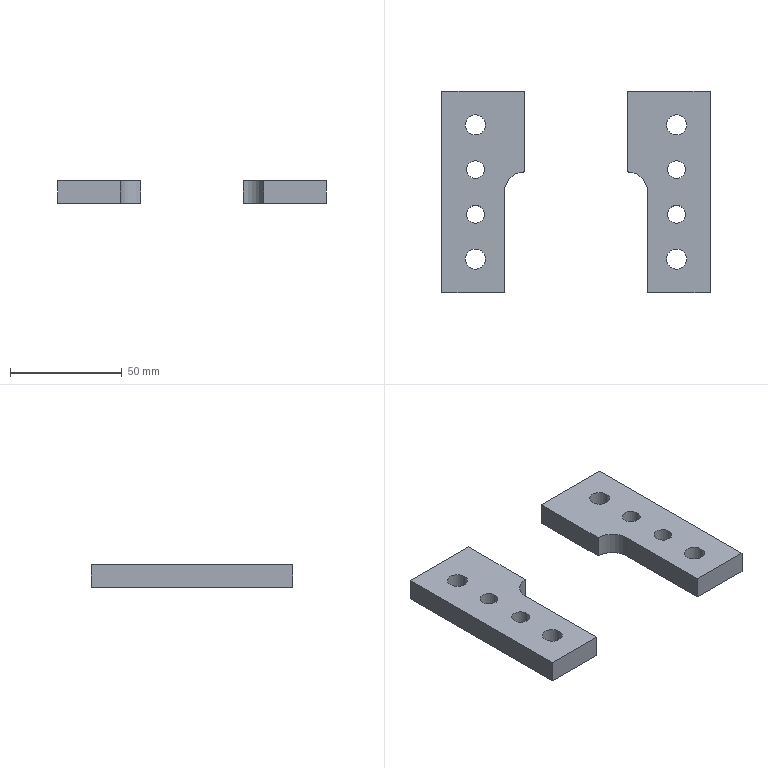Part | NX | features DATUM_CSYS 1, EXTRUDE 1 | 2 solids | 24 faces | box 120 x 90 x 10 mm | volume 52672 mm3 | plane 14 | cylinder 10 | commonest cylinder face diameters 8 x4 9 x4 18 x2
STEP:
#1=CARTESIAN_POINT('',(23.,9.,0.));
#2=VERTEX_POINT('',#1);
#3=CARTESIAN_POINT('',(23.,45.,0.));
#4=VERTEX_POINT('',#3);
#5=CARTESIAN_POINT('',(23.,9.,0.));
#6=DIRECTION('',(0.,1.,0.));
#7=VECTOR('',#6,1000.);
#8=LINE('',#5,#7);
#9=EDGE_CURVE('',#2,#4,#8,.T.);
#10=ORIENTED_EDGE('',*,*,#9,.F.);
#11=CARTESIAN_POINT('',(23.,9.,10.));
#12=VERTEX_POINT('',#11);
#13=CARTESIAN_POINT('',(23.,9.,10.));
#14=DIRECTION('',(0.,0.,-1.));
#15=VECTOR('',#14,1000.);
#16=LINE('',#13,#15);
#17=EDGE_CURVE('',#12,#2,#16,.T.);
#18=ORIENTED_EDGE('',*,*,#17,.F.);
#19=CARTESIAN_POINT('',(23.,45.,10.));
#20=VERTEX_POINT('',#19);
#21=CARTESIAN_POINT('',(23.,9.,10.));
#22=DIRECTION('',(0.,1.,0.));
#23=VECTOR('',#22,1000.);
#24=LINE('',#21,#23);
#25=EDGE_CURVE('',#12,#20,#24,.T.);
#26=ORIENTED_EDGE('',*,*,#25,.T.);
#27=CARTESIAN_POINT('',(23.,45.,10.));
#28=DIRECTION('',(0.,0.,-1.));
#29=VECTOR('',#28,1000.);
#30=LINE('',#27,#29);
#31=EDGE_CURVE('',#20,#4,#30,.T.);
#32=ORIENTED_EDGE('',*,*,#31,.T.);
#33=EDGE_LOOP('',(#10,#18,#26,#32));
#34=FACE_BOUND('',#33,.T.);
#35=CARTESIAN_POINT('',(23.,9.,10.));
#36=DIRECTION('',(-1.,0.,0.));
#37=DIRECTION('',(0.,0.,1.));
#38=AXIS2_PLACEMENT_3D('',#35,#36,#37);
#39=PLANE('',#38);
#40=ADVANCED_FACE('',(#34),#39,.T.);
#41=CARTESIAN_POINT('',(60.,45.,0.));
#42=VERTEX_POINT('',#41);
#43=CARTESIAN_POINT('',(23.,45.,0.));
#44=DIRECTION('',(1.,0.,0.));
#45=VECTOR('',#44,1000.);
#46=LINE('',#43,#45);
#47=EDGE_CURVE('',#4,#42,#46,.T.);
#48=ORIENTED_EDGE('',*,*,#47,.F.);
#49=ORIENTED_EDGE('',*,*,#31,.F.);
#50=CARTESIAN_POINT('',(60.,45.,10.));
#51=VERTEX_POINT('',#50);
#52=CARTESIAN_POINT('',(23.,45.,10.));
#53=DIRECTION('',(1.,0.,0.));
#54=VECTOR('',#53,1000.);
#55=LINE('',#52,#54);
#56=EDGE_CURVE('',#20,#51,#55,.T.);
#57=ORIENTED_EDGE('',*,*,#56,.T.);
#58=CARTESIAN_POINT('',(60.,45.,10.));
#59=DIRECTION('',(0.,0.,-1.));
#60=VECTOR('',#59,1000.);
#61=LINE('',#58,#60);
#62=EDGE_CURVE('',#51,#42,#61,.T.);
#63=ORIENTED_EDGE('',*,*,#62,.T.);
#64=EDGE_LOOP('',(#48,#49,#57,#63));
#65=FACE_BOUND('',#64,.T.);
#66=CARTESIAN_POINT('',(23.,45.,10.));
#67=DIRECTION('',(0.,1.,0.));
#68=DIRECTION('',(0.,0.,1.));
#69=AXIS2_PLACEMENT_3D('',#66,#67,#68);
#70=PLANE('',#69);
#71=ADVANCED_FACE('',(#65),#70,.T.);
#72=CARTESIAN_POINT('',(60.,-45.,0.));
#73=VERTEX_POINT('',#72);
#74=CARTESIAN_POINT('',(60.,45.,0.));
#75=DIRECTION('',(0.,-1.,0.));
#76=VECTOR('',#75,1000.);
#77=LINE('',#74,#76);
#78=EDGE_CURVE('',#42,#73,#77,.T.);
#79=ORIENTED_EDGE('',*,*,#78,.F.);
#80=ORIENTED_EDGE('',*,*,#62,.F.);
#81=CARTESIAN_POINT('',(60.,-45.,10.));
#82=VERTEX_POINT('',#81);
#83=CARTESIAN_POINT('',(60.,45.,10.));
#84=DIRECTION('',(0.,-1.,0.));
#85=VECTOR('',#84,1000.);
#86=LINE('',#83,#85);
#87=EDGE_CURVE('',#51,#82,#86,.T.);
#88=ORIENTED_EDGE('',*,*,#87,.T.);
#89=CARTESIAN_POINT('',(60.,-45.,10.));
#90=DIRECTION('',(0.,0.,-1.));
#91=VECTOR('',#90,1000.);
#92=LINE('',#89,#91);
#93=EDGE_CURVE('',#82,#73,#92,.T.);
#94=ORIENTED_EDGE('',*,*,#93,.T.);
#95=EDGE_LOOP('',(#79,#80,#88,#94));
#96=FACE_BOUND('',#95,.T.);
#97=CARTESIAN_POINT('',(60.,45.,10.));
#98=DIRECTION('',(1.,0.,0.));
#99=DIRECTION('',(0.,0.,-1.));
#100=AXIS2_PLACEMENT_3D('',#97,#98,#99);
#101=PLANE('',#100);
#102=ADVANCED_FACE('',(#96),#101,.T.);
#103=CARTESIAN_POINT('',(32.,-45.,0.));
#104=VERTEX_POINT('',#103);
#105=CARTESIAN_POINT('',(60.,-45.,0.));
#106=DIRECTION('',(-1.,0.,0.));
#107=VECTOR('',#106,1000.);
#108=LINE('',#105,#107);
#109=EDGE_CURVE('',#73,#104,#108,.T.);
#110=ORIENTED_EDGE('',*,*,#109,.F.);
#111=ORIENTED_EDGE('',*,*,#93,.F.);
#112=CARTESIAN_POINT('',(32.,-45.,10.));
#113=VERTEX_POINT('',#112);
#114=CARTESIAN_POINT('',(60.,-45.,10.));
#115=DIRECTION('',(-1.,0.,0.));
#116=VECTOR('',#115,1000.);
#117=LINE('',#114,#116);
#118=EDGE_CURVE('',#82,#113,#117,.T.);
#119=ORIENTED_EDGE('',*,*,#118,.T.);
#120=CARTESIAN_POINT('',(32.,-45.,10.));
#121=DIRECTION('',(0.,0.,-1.));
#122=VECTOR('',#121,1000.);
#123=LINE('',#120,#122);
#124=EDGE_CURVE('',#113,#104,#123,.T.);
#125=ORIENTED_EDGE('',*,*,#124,.T.);
#126=EDGE_LOOP('',(#110,#111,#119,#125));
#127=FACE_BOUND('',#126,.T.);
#128=CARTESIAN_POINT('',(60.,-45.,10.));
#129=DIRECTION('',(0.,-1.,0.));
#130=DIRECTION('',(0.,0.,-1.));
#131=AXIS2_PLACEMENT_3D('',#128,#129,#130);
#132=PLANE('',#131);
#133=ADVANCED_FACE('',(#127),#132,.T.);
#134=CARTESIAN_POINT('',(32.,0.,0.));
#135=VERTEX_POINT('',#134);
#136=CARTESIAN_POINT('',(32.,-45.,0.));
#137=DIRECTION('',(0.,1.,0.));
#138=VECTOR('',#137,1000.);
#139=LINE('',#136,#138);
#140=EDGE_CURVE('',#104,#135,#139,.T.);
#141=ORIENTED_EDGE('',*,*,#140,.F.);
#142=ORIENTED_EDGE('',*,*,#124,.F.);
#143=CARTESIAN_POINT('',(32.,0.,10.));
#144=VERTEX_POINT('',#143);
#145=CARTESIAN_POINT('',(32.,-45.,10.));
#146=DIRECTION('',(0.,1.,0.));
#147=VECTOR('',#146,1000.);
#148=LINE('',#145,#147);
#149=EDGE_CURVE('',#113,#144,#148,.T.);
#150=ORIENTED_EDGE('',*,*,#149,.T.);
#151=CARTESIAN_POINT('',(32.,0.,10.));
#152=DIRECTION('',(0.,0.,-1.));
#153=VECTOR('',#152,1000.);
#154=LINE('',#151,#153);
#155=EDGE_CURVE('',#144,#135,#154,.T.);
#156=ORIENTED_EDGE('',*,*,#155,.T.);
#157=EDGE_LOOP('',(#141,#142,#150,#156));
#158=FACE_BOUND('',#157,.T.);
#159=CARTESIAN_POINT('',(32.,-45.,10.));
#160=DIRECTION('',(-1.,0.,0.));
#161=DIRECTION('',(0.,0.,1.));
#162=AXIS2_PLACEMENT_3D('',#159,#160,#161);
#163=PLANE('',#162);
#164=ADVANCED_FACE('',(#158),#163,.T.);
#165=CARTESIAN_POINT('',(49.5,30.,10.));
#166=VERTEX_POINT('',#165);
#167=CARTESIAN_POINT('',(45.,30.,10.));
#168=DIRECTION('',(0.,0.,1.));
#169=DIRECTION('',(1.,0.,0.));
#170=AXIS2_PLACEMENT_3D('',#167,#168,#169);
#171=CIRCLE('',#170,4.5);
#172=EDGE_CURVE('',#166,#166,#171,.T.);
#173=ORIENTED_EDGE('',*,*,#172,.T.);
#174=EDGE_LOOP('',(#173));
#175=FACE_BOUND('',#174,.T.);
#176=CARTESIAN_POINT('',(49.5,30.,0.));
#177=VERTEX_POINT('',#176);
#178=CARTESIAN_POINT('',(45.,30.,0.));
#179=DIRECTION('',(0.,0.,1.));
#180=DIRECTION('',(1.,0.,0.));
#181=AXIS2_PLACEMENT_3D('',#178,#179,#180);
#182=CIRCLE('',#181,4.5);
#183=EDGE_CURVE('',#177,#177,#182,.T.);
#184=ORIENTED_EDGE('',*,*,#183,.F.);
#185=EDGE_LOOP('',(#184));
#186=FACE_BOUND('',#185,.T.);
#187=CARTESIAN_POINT('',(45.,30.,10.));
#188=DIRECTION('',(0.,0.,-1.));
#189=DIRECTION('',(-1.,0.,0.));
#190=AXIS2_PLACEMENT_3D('',#187,#188,#189);
#191=CYLINDRICAL_SURFACE('',#190,4.5);
#192=ADVANCED_FACE('',(#175,#186),#191,.F.);
#193=CARTESIAN_POINT('',(49.,-10.,10.));
#194=VERTEX_POINT('',#193);
#195=CARTESIAN_POINT('',(45.,-10.,10.));
#196=DIRECTION('',(0.,0.,1.));
#197=DIRECTION('',(1.,0.,0.));
#198=AXIS2_PLACEMENT_3D('',#195,#196,#197);
#199=CIRCLE('',#198,4.);
#200=EDGE_CURVE('',#194,#194,#199,.T.);
#201=ORIENTED_EDGE('',*,*,#200,.T.);
#202=EDGE_LOOP('',(#201));
#203=FACE_BOUND('',#202,.T.);
#204=CARTESIAN_POINT('',(49.,-10.,0.));
#205=VERTEX_POINT('',#204);
#206=CARTESIAN_POINT('',(45.,-10.,0.));
#207=DIRECTION('',(0.,0.,1.));
#208=DIRECTION('',(1.,0.,0.));
#209=AXIS2_PLACEMENT_3D('',#206,#207,#208);
#210=CIRCLE('',#209,4.);
#211=EDGE_CURVE('',#205,#205,#210,.T.);
#212=ORIENTED_EDGE('',*,*,#211,.F.);
#213=EDGE_LOOP('',(#212));
#214=FACE_BOUND('',#213,.T.);
#215=CARTESIAN_POINT('',(45.,-10.,10.));
#216=DIRECTION('',(0.,0.,-1.));
#217=DIRECTION('',(-1.,0.,0.));
#218=AXIS2_PLACEMENT_3D('',#215,#216,#217);
#219=CYLINDRICAL_SURFACE('',#218,4.);
#220=ADVANCED_FACE('',(#203,#214),#219,.F.);
#221=CARTESIAN_POINT('',(49.,10.,10.));
#222=VERTEX_POINT('',#221);
#223=CARTESIAN_POINT('',(45.,10.,10.));
#224=DIRECTION('',(0.,0.,1.));
#225=DIRECTION('',(1.,0.,0.));
#226=AXIS2_PLACEMENT_3D('',#223,#224,#225);
#227=CIRCLE('',#226,4.);
#228=EDGE_CURVE('',#222,#222,#227,.T.);
#229=ORIENTED_EDGE('',*,*,#228,.T.);
#230=EDGE_LOOP('',(#229));
#231=FACE_BOUND('',#230,.T.);
#232=CARTESIAN_POINT('',(49.,10.,0.));
#233=VERTEX_POINT('',#232);
#234=CARTESIAN_POINT('',(45.,10.,0.));
#235=DIRECTION('',(0.,0.,1.));
#236=DIRECTION('',(1.,0.,0.));
#237=AXIS2_PLACEMENT_3D('',#234,#235,#236);
#238=CIRCLE('',#237,4.);
#239=EDGE_CURVE('',#233,#233,#238,.T.);
#240=ORIENTED_EDGE('',*,*,#239,.F.);
#241=EDGE_LOOP('',(#240));
#242=FACE_BOUND('',#241,.T.);
#243=CARTESIAN_POINT('',(45.,10.,10.));
#244=DIRECTION('',(0.,0.,-1.));
#245=DIRECTION('',(-1.,0.,0.));
#246=AXIS2_PLACEMENT_3D('',#243,#244,#245);
#247=CYLINDRICAL_SURFACE('',#246,4.);
#248=ADVANCED_FACE('',(#231,#242),#247,.F.);
#249=CARTESIAN_POINT('',(23.,0.,0.));
#250=DIRECTION('',(0.,0.,1.));
#251=DIRECTION('',(1.,0.,0.));
#252=AXIS2_PLACEMENT_3D('',#249,#250,#251);
#253=CIRCLE('',#252,9.);
#254=EDGE_CURVE('',#135,#2,#253,.T.);
#255=ORIENTED_EDGE('',*,*,#254,.F.);
#256=ORIENTED_EDGE('',*,*,#155,.F.);
#257=CARTESIAN_POINT('',(23.,0.,10.));
#258=DIRECTION('',(0.,0.,1.));
#259=DIRECTION('',(1.,0.,0.));
#260=AXIS2_PLACEMENT_3D('',#257,#258,#259);
#261=CIRCLE('',#260,9.);
#262=EDGE_CURVE('',#144,#12,#261,.T.);
#263=ORIENTED_EDGE('',*,*,#262,.T.);
#264=ORIENTED_EDGE('',*,*,#17,.T.);
#265=EDGE_LOOP('',(#255,#256,#263,#264));
#266=FACE_BOUND('',#265,.T.);
#267=CARTESIAN_POINT('',(23.,0.,10.));
#268=DIRECTION('',(0.,0.,-1.));
#269=DIRECTION('',(-1.,0.,0.));
#270=AXIS2_PLACEMENT_3D('',#267,#268,#269);
#271=CYLINDRICAL_SURFACE('',#270,9.);
#272=ADVANCED_FACE('',(#266),#271,.F.);
#273=CARTESIAN_POINT('',(49.5,-30.,10.));
#274=VERTEX_POINT('',#273);
#275=CARTESIAN_POINT('',(45.,-30.,10.));
#276=DIRECTION('',(0.,0.,1.));
#277=DIRECTION('',(1.,0.,0.));
#278=AXIS2_PLACEMENT_3D('',#275,#276,#277);
#279=CIRCLE('',#278,4.5);
#280=EDGE_CURVE('',#274,#274,#279,.T.);
#281=ORIENTED_EDGE('',*,*,#280,.T.);
#282=EDGE_LOOP('',(#281));
#283=FACE_BOUND('',#282,.T.);
#284=CARTESIAN_POINT('',(49.5,-30.,0.));
#285=VERTEX_POINT('',#284);
#286=CARTESIAN_POINT('',(45.,-30.,0.));
#287=DIRECTION('',(0.,0.,1.));
#288=DIRECTION('',(1.,0.,0.));
#289=AXIS2_PLACEMENT_3D('',#286,#287,#288);
#290=CIRCLE('',#289,4.5);
#291=EDGE_CURVE('',#285,#285,#290,.T.);
#292=ORIENTED_EDGE('',*,*,#291,.F.);
#293=EDGE_LOOP('',(#292));
#294=FACE_BOUND('',#293,.T.);
#295=CARTESIAN_POINT('',(45.,-30.,10.));
#296=DIRECTION('',(0.,0.,-1.));
#297=DIRECTION('',(-1.,0.,0.));
#298=AXIS2_PLACEMENT_3D('',#295,#296,#297);
#299=CYLINDRICAL_SURFACE('',#298,4.5);
#300=ADVANCED_FACE('',(#283,#294),#299,.F.);
#301=ORIENTED_EDGE('',*,*,#25,.F.);
#302=ORIENTED_EDGE('',*,*,#262,.F.);
#303=ORIENTED_EDGE('',*,*,#149,.F.);
#304=ORIENTED_EDGE('',*,*,#118,.F.);
#305=ORIENTED_EDGE('',*,*,#87,.F.);
#306=ORIENTED_EDGE('',*,*,#56,.F.);
#307=EDGE_LOOP('',(#301,#302,#303,#304,#305,#306));
#308=FACE_BOUND('',#307,.T.);
#309=ORIENTED_EDGE('',*,*,#228,.F.);
#310=EDGE_LOOP('',(#309));
#311=FACE_BOUND('',#310,.T.);
#312=ORIENTED_EDGE('',*,*,#200,.F.);
#313=EDGE_LOOP('',(#312));
#314=FACE_BOUND('',#313,.T.);
#315=ORIENTED_EDGE('',*,*,#172,.F.);
#316=EDGE_LOOP('',(#315));
#317=FACE_BOUND('',#316,.T.);
#318=ORIENTED_EDGE('',*,*,#280,.F.);
#319=EDGE_LOOP('',(#318));
#320=FACE_BOUND('',#319,.T.);
#321=CARTESIAN_POINT('',(23.,0.,10.));
#322=DIRECTION('',(0.,0.,1.));
#323=DIRECTION('',(1.,0.,0.));
#324=AXIS2_PLACEMENT_3D('',#321,#322,#323);
#325=PLANE('',#324);
#326=ADVANCED_FACE('',(#308,#311,#314,#317,#320),#325,.T.);
#327=ORIENTED_EDGE('',*,*,#9,.T.);
#328=ORIENTED_EDGE('',*,*,#47,.T.);
#329=ORIENTED_EDGE('',*,*,#78,.T.);
#330=ORIENTED_EDGE('',*,*,#109,.T.);
#331=ORIENTED_EDGE('',*,*,#140,.T.);
#332=ORIENTED_EDGE('',*,*,#254,.T.);
#333=EDGE_LOOP('',(#327,#328,#329,#330,#331,#332));
#334=FACE_BOUND('',#333,.T.);
#335=ORIENTED_EDGE('',*,*,#239,.T.);
#336=EDGE_LOOP('',(#335));
#337=FACE_BOUND('',#336,.T.);
#338=ORIENTED_EDGE('',*,*,#211,.T.);
#339=EDGE_LOOP('',(#338));
#340=FACE_BOUND('',#339,.T.);
#341=ORIENTED_EDGE('',*,*,#183,.T.);
#342=EDGE_LOOP('',(#341));
#343=FACE_BOUND('',#342,.T.);
#344=ORIENTED_EDGE('',*,*,#291,.T.);
#345=EDGE_LOOP('',(#344));
#346=FACE_BOUND('',#345,.T.);
#347=CARTESIAN_POINT('',(23.,0.,0.));
#348=DIRECTION('',(0.,0.,1.));
#349=DIRECTION('',(1.,0.,0.));
#350=AXIS2_PLACEMENT_3D('',#347,#348,#349);
#351=PLANE('',#350);
#352=ADVANCED_FACE('',(#334,#337,#340,#343,#346),#351,.F.);
#353=CLOSED_SHELL('',(#40,#71,#102,#133,#164,#192,#220,#248,#272,#300,#326,#352));
#354=MANIFOLD_SOLID_BREP('',#353);
#355=CARTESIAN_POINT('',(-60.,45.,0.));
#356=VERTEX_POINT('',#355);
#357=CARTESIAN_POINT('',(-60.,-45.,0.));
#358=VERTEX_POINT('',#357);
#359=CARTESIAN_POINT('',(-60.,45.,0.));
#360=DIRECTION('',(0.,-1.,0.));
#361=VECTOR('',#360,1000.);
#362=LINE('',#359,#361);
#363=EDGE_CURVE('',#356,#358,#362,.T.);
#364=ORIENTED_EDGE('',*,*,#363,.T.);
#365=CARTESIAN_POINT('',(-60.,-45.,10.));
#366=VERTEX_POINT('',#365);
#367=CARTESIAN_POINT('',(-60.,-45.,10.));
#368=DIRECTION('',(0.,0.,-1.));
#369=VECTOR('',#368,1000.);
#370=LINE('',#367,#369);
#371=EDGE_CURVE('',#366,#358,#370,.T.);
#372=ORIENTED_EDGE('',*,*,#371,.F.);
#373=CARTESIAN_POINT('',(-60.,45.,10.));
#374=VERTEX_POINT('',#373);
#375=CARTESIAN_POINT('',(-60.,45.,10.));
#376=DIRECTION('',(0.,-1.,0.));
#377=VECTOR('',#376,1000.);
#378=LINE('',#375,#377);
#379=EDGE_CURVE('',#374,#366,#378,.T.);
#380=ORIENTED_EDGE('',*,*,#379,.F.);
#381=CARTESIAN_POINT('',(-60.,45.,10.));
#382=DIRECTION('',(0.,0.,-1.));
#383=VECTOR('',#382,1000.);
#384=LINE('',#381,#383);
#385=EDGE_CURVE('',#374,#356,#384,.T.);
#386=ORIENTED_EDGE('',*,*,#385,.T.);
#387=EDGE_LOOP('',(#364,#372,#380,#386));
#388=FACE_BOUND('',#387,.T.);
#389=CARTESIAN_POINT('',(-60.,45.,10.));
#390=DIRECTION('',(1.,0.,0.));
#391=DIRECTION('',(0.,0.,-1.));
#392=AXIS2_PLACEMENT_3D('',#389,#390,#391);
#393=PLANE('',#392);
#394=ADVANCED_FACE('',(#388),#393,.F.);
#395=CARTESIAN_POINT('',(-32.,-45.,0.));
#396=VERTEX_POINT('',#395);
#397=CARTESIAN_POINT('',(-60.,-45.,0.));
#398=DIRECTION('',(1.,0.,0.));
#399=VECTOR('',#398,1000.);
#400=LINE('',#397,#399);
#401=EDGE_CURVE('',#358,#396,#400,.T.);
#402=ORIENTED_EDGE('',*,*,#401,.T.);
#403=CARTESIAN_POINT('',(-32.,-45.,10.));
#404=VERTEX_POINT('',#403);
#405=CARTESIAN_POINT('',(-32.,-45.,10.));
#406=DIRECTION('',(0.,0.,-1.));
#407=VECTOR('',#406,1000.);
#408=LINE('',#405,#407);
#409=EDGE_CURVE('',#404,#396,#408,.T.);
#410=ORIENTED_EDGE('',*,*,#409,.F.);
#411=CARTESIAN_POINT('',(-60.,-45.,10.));
#412=DIRECTION('',(1.,0.,0.));
#413=VECTOR('',#412,1000.);
#414=LINE('',#411,#413);
#415=EDGE_CURVE('',#366,#404,#414,.T.);
#416=ORIENTED_EDGE('',*,*,#415,.F.);
#417=ORIENTED_EDGE('',*,*,#371,.T.);
#418=EDGE_LOOP('',(#402,#410,#416,#417));
#419=FACE_BOUND('',#418,.T.);
#420=CARTESIAN_POINT('',(-60.,-45.,10.));
#421=DIRECTION('',(0.,1.,0.));
#422=DIRECTION('',(0.,0.,1.));
#423=AXIS2_PLACEMENT_3D('',#420,#421,#422);
#424=PLANE('',#423);
#425=ADVANCED_FACE('',(#419),#424,.F.);
#426=CARTESIAN_POINT('',(-32.,0.,0.));
#427=VERTEX_POINT('',#426);
#428=CARTESIAN_POINT('',(-32.,-45.,0.));
#429=DIRECTION('',(0.,1.,0.));
#430=VECTOR('',#429,1000.);
#431=LINE('',#428,#430);
#432=EDGE_CURVE('',#396,#427,#431,.T.);
#433=ORIENTED_EDGE('',*,*,#432,.T.);
#434=CARTESIAN_POINT('',(-32.,0.,10.));
#435=VERTEX_POINT('',#434);
#436=CARTESIAN_POINT('',(-32.,0.,10.));
#437=DIRECTION('',(0.,0.,-1.));
#438=VECTOR('',#437,1000.);
#439=LINE('',#436,#438);
#440=EDGE_CURVE('',#435,#427,#439,.T.);
#441=ORIENTED_EDGE('',*,*,#440,.F.);
#442=CARTESIAN_POINT('',(-32.,-45.,10.));
#443=DIRECTION('',(0.,1.,0.));
#444=VECTOR('',#443,1000.);
#445=LINE('',#442,#444);
#446=EDGE_CURVE('',#404,#435,#445,.T.);
#447=ORIENTED_EDGE('',*,*,#446,.F.);
#448=ORIENTED_EDGE('',*,*,#409,.T.);
#449=EDGE_LOOP('',(#433,#441,#447,#448));
#450=FACE_BOUND('',#449,.T.);
#451=CARTESIAN_POINT('',(-32.,-45.,10.));
#452=DIRECTION('',(-1.,0.,0.));
#453=DIRECTION('',(0.,0.,1.));
#454=AXIS2_PLACEMENT_3D('',#451,#452,#453);
#455=PLANE('',#454);
#456=ADVANCED_FACE('',(#450),#455,.F.);
#457=CARTESIAN_POINT('',(-23.,9.,0.));
#458=VERTEX_POINT('',#457);
#459=CARTESIAN_POINT('',(-23.,0.,0.));
#460=DIRECTION('',(0.,0.,-1.));
#461=DIRECTION('',(1.,0.,0.));
#462=AXIS2_PLACEMENT_3D('',#459,#460,#461);
#463=CIRCLE('',#462,9.);
#464=EDGE_CURVE('',#427,#458,#463,.T.);
#465=ORIENTED_EDGE('',*,*,#464,.T.);
#466=CARTESIAN_POINT('',(-23.,9.,10.));
#467=VERTEX_POINT('',#466);
#468=CARTESIAN_POINT('',(-23.,9.,10.));
#469=DIRECTION('',(0.,0.,-1.));
#470=VECTOR('',#469,1000.);
#471=LINE('',#468,#470);
#472=EDGE_CURVE('',#467,#458,#471,.T.);
#473=ORIENTED_EDGE('',*,*,#472,.F.);
#474=CARTESIAN_POINT('',(-23.,0.,10.));
#475=DIRECTION('',(0.,0.,-1.));
#476=DIRECTION('',(1.,0.,0.));
#477=AXIS2_PLACEMENT_3D('',#474,#475,#476);
#478=CIRCLE('',#477,9.);
#479=EDGE_CURVE('',#435,#467,#478,.T.);
#480=ORIENTED_EDGE('',*,*,#479,.F.);
#481=ORIENTED_EDGE('',*,*,#440,.T.);
#482=EDGE_LOOP('',(#465,#473,#480,#481));
#483=FACE_BOUND('',#482,.T.);
#484=CARTESIAN_POINT('',(-23.,0.,10.));
#485=DIRECTION('',(0.,0.,-1.));
#486=DIRECTION('',(-1.,0.,0.));
#487=AXIS2_PLACEMENT_3D('',#484,#485,#486);
#488=CYLINDRICAL_SURFACE('',#487,9.);
#489=ADVANCED_FACE('',(#483),#488,.F.);
#490=CARTESIAN_POINT('',(-23.,45.,0.));
#491=VERTEX_POINT('',#490);
#492=CARTESIAN_POINT('',(-23.,9.,0.));
#493=DIRECTION('',(0.,1.,0.));
#494=VECTOR('',#493,1000.);
#495=LINE('',#492,#494);
#496=EDGE_CURVE('',#458,#491,#495,.T.);
#497=ORIENTED_EDGE('',*,*,#496,.T.);
#498=CARTESIAN_POINT('',(-23.,45.,10.));
#499=VERTEX_POINT('',#498);
#500=CARTESIAN_POINT('',(-23.,45.,10.));
#501=DIRECTION('',(0.,0.,-1.));
#502=VECTOR('',#501,1000.);
#503=LINE('',#500,#502);
#504=EDGE_CURVE('',#499,#491,#503,.T.);
#505=ORIENTED_EDGE('',*,*,#504,.F.);
#506=CARTESIAN_POINT('',(-23.,9.,10.));
#507=DIRECTION('',(0.,1.,0.));
#508=VECTOR('',#507,1000.);
#509=LINE('',#506,#508);
#510=EDGE_CURVE('',#467,#499,#509,.T.);
#511=ORIENTED_EDGE('',*,*,#510,.F.);
#512=ORIENTED_EDGE('',*,*,#472,.T.);
#513=EDGE_LOOP('',(#497,#505,#511,#512));
#514=FACE_BOUND('',#513,.T.);
#515=CARTESIAN_POINT('',(-23.,9.,10.));
#516=DIRECTION('',(-1.,0.,0.));
#517=DIRECTION('',(0.,0.,1.));
#518=AXIS2_PLACEMENT_3D('',#515,#516,#517);
#519=PLANE('',#518);
#520=ADVANCED_FACE('',(#514),#519,.F.);
#521=CARTESIAN_POINT('',(-41.,-10.,10.));
#522=VERTEX_POINT('',#521);
#523=CARTESIAN_POINT('',(-45.,-10.,10.));
#524=DIRECTION('',(0.,0.,1.));
#525=DIRECTION('',(1.,0.,0.));
#526=AXIS2_PLACEMENT_3D('',#523,#524,#525);
#527=CIRCLE('',#526,4.);
#528=EDGE_CURVE('',#522,#522,#527,.T.);
#529=ORIENTED_EDGE('',*,*,#528,.T.);
#530=EDGE_LOOP('',(#529));
#531=FACE_BOUND('',#530,.T.);
#532=CARTESIAN_POINT('',(-41.,-10.,0.));
#533=VERTEX_POINT('',#532);
#534=CARTESIAN_POINT('',(-45.,-10.,0.));
#535=DIRECTION('',(0.,0.,1.));
#536=DIRECTION('',(1.,0.,0.));
#537=AXIS2_PLACEMENT_3D('',#534,#535,#536);
#538=CIRCLE('',#537,4.);
#539=EDGE_CURVE('',#533,#533,#538,.T.);
#540=ORIENTED_EDGE('',*,*,#539,.F.);
#541=EDGE_LOOP('',(#540));
#542=FACE_BOUND('',#541,.T.);
#543=CARTESIAN_POINT('',(-45.,-10.,10.));
#544=DIRECTION('',(0.,0.,-1.));
#545=DIRECTION('',(-1.,0.,0.));
#546=AXIS2_PLACEMENT_3D('',#543,#544,#545);
#547=CYLINDRICAL_SURFACE('',#546,4.);
#548=ADVANCED_FACE('',(#531,#542),#547,.F.);
#549=CARTESIAN_POINT('',(-40.5,30.,10.));
#550=VERTEX_POINT('',#549);
#551=CARTESIAN_POINT('',(-45.,30.,10.));
#552=DIRECTION('',(0.,0.,1.));
#553=DIRECTION('',(1.,0.,0.));
#554=AXIS2_PLACEMENT_3D('',#551,#552,#553);
#555=CIRCLE('',#554,4.5);
#556=EDGE_CURVE('',#550,#550,#555,.T.);
#557=ORIENTED_EDGE('',*,*,#556,.T.);
#558=EDGE_LOOP('',(#557));
#559=FACE_BOUND('',#558,.T.);
#560=CARTESIAN_POINT('',(-40.5,30.,0.));
#561=VERTEX_POINT('',#560);
#562=CARTESIAN_POINT('',(-45.,30.,0.));
#563=DIRECTION('',(0.,0.,1.));
#564=DIRECTION('',(1.,0.,0.));
#565=AXIS2_PLACEMENT_3D('',#562,#563,#564);
#566=CIRCLE('',#565,4.5);
#567=EDGE_CURVE('',#561,#561,#566,.T.);
#568=ORIENTED_EDGE('',*,*,#567,.F.);
#569=EDGE_LOOP('',(#568));
#570=FACE_BOUND('',#569,.T.);
#571=CARTESIAN_POINT('',(-45.,30.,10.));
#572=DIRECTION('',(0.,0.,-1.));
#573=DIRECTION('',(-1.,0.,0.));
#574=AXIS2_PLACEMENT_3D('',#571,#572,#573);
#575=CYLINDRICAL_SURFACE('',#574,4.5);
#576=ADVANCED_FACE('',(#559,#570),#575,.F.);
#577=CARTESIAN_POINT('',(-40.5,-30.,10.));
#578=VERTEX_POINT('',#577);
#579=CARTESIAN_POINT('',(-45.,-30.,10.));
#580=DIRECTION('',(0.,0.,1.));
#581=DIRECTION('',(1.,0.,0.));
#582=AXIS2_PLACEMENT_3D('',#579,#580,#581);
#583=CIRCLE('',#582,4.5);
#584=EDGE_CURVE('',#578,#578,#583,.T.);
#585=ORIENTED_EDGE('',*,*,#584,.T.);
#586=EDGE_LOOP('',(#585));
#587=FACE_BOUND('',#586,.T.);
#588=CARTESIAN_POINT('',(-40.5,-30.,0.));
#589=VERTEX_POINT('',#588);
#590=CARTESIAN_POINT('',(-45.,-30.,0.));
#591=DIRECTION('',(0.,0.,1.));
#592=DIRECTION('',(1.,0.,0.));
#593=AXIS2_PLACEMENT_3D('',#590,#591,#592);
#594=CIRCLE('',#593,4.5);
#595=EDGE_CURVE('',#589,#589,#594,.T.);
#596=ORIENTED_EDGE('',*,*,#595,.F.);
#597=EDGE_LOOP('',(#596));
#598=FACE_BOUND('',#597,.T.);
#599=CARTESIAN_POINT('',(-45.,-30.,10.));
#600=DIRECTION('',(0.,0.,-1.));
#601=DIRECTION('',(-1.,0.,0.));
#602=AXIS2_PLACEMENT_3D('',#599,#600,#601);
#603=CYLINDRICAL_SURFACE('',#602,4.5);
#604=ADVANCED_FACE('',(#587,#598),#603,.F.);
#605=CARTESIAN_POINT('',(-23.,45.,0.));
#606=DIRECTION('',(-1.,0.,0.));
#607=VECTOR('',#606,1000.);
#608=LINE('',#605,#607);
#609=EDGE_CURVE('',#491,#356,#608,.T.);
#610=ORIENTED_EDGE('',*,*,#609,.T.);
#611=ORIENTED_EDGE('',*,*,#385,.F.);
#612=CARTESIAN_POINT('',(-23.,45.,10.));
#613=DIRECTION('',(-1.,0.,0.));
#614=VECTOR('',#613,1000.);
#615=LINE('',#612,#614);
#616=EDGE_CURVE('',#499,#374,#615,.T.);
#617=ORIENTED_EDGE('',*,*,#616,.F.);
#618=ORIENTED_EDGE('',*,*,#504,.T.);
#619=EDGE_LOOP('',(#610,#611,#617,#618));
#620=FACE_BOUND('',#619,.T.);
#621=CARTESIAN_POINT('',(-23.,45.,10.));
#622=DIRECTION('',(0.,-1.,0.));
#623=DIRECTION('',(0.,0.,-1.));
#624=AXIS2_PLACEMENT_3D('',#621,#622,#623);
#625=PLANE('',#624);
#626=ADVANCED_FACE('',(#620),#625,.F.);
#627=CARTESIAN_POINT('',(-41.,10.,10.));
#628=VERTEX_POINT('',#627);
#629=CARTESIAN_POINT('',(-45.,10.,10.));
#630=DIRECTION('',(0.,0.,1.));
#631=DIRECTION('',(1.,0.,0.));
#632=AXIS2_PLACEMENT_3D('',#629,#630,#631);
#633=CIRCLE('',#632,4.);
#634=EDGE_CURVE('',#628,#628,#633,.T.);
#635=ORIENTED_EDGE('',*,*,#634,.T.);
#636=EDGE_LOOP('',(#635));
#637=FACE_BOUND('',#636,.T.);
#638=CARTESIAN_POINT('',(-41.,10.,0.));
#639=VERTEX_POINT('',#638);
#640=CARTESIAN_POINT('',(-45.,10.,0.));
#641=DIRECTION('',(0.,0.,1.));
#642=DIRECTION('',(1.,0.,0.));
#643=AXIS2_PLACEMENT_3D('',#640,#641,#642);
#644=CIRCLE('',#643,4.);
#645=EDGE_CURVE('',#639,#639,#644,.T.);
#646=ORIENTED_EDGE('',*,*,#645,.F.);
#647=EDGE_LOOP('',(#646));
#648=FACE_BOUND('',#647,.T.);
#649=CARTESIAN_POINT('',(-45.,10.,10.));
#650=DIRECTION('',(0.,0.,-1.));
#651=DIRECTION('',(-1.,0.,0.));
#652=AXIS2_PLACEMENT_3D('',#649,#650,#651);
#653=CYLINDRICAL_SURFACE('',#652,4.);
#654=ADVANCED_FACE('',(#637,#648),#653,.F.);
#655=ORIENTED_EDGE('',*,*,#379,.T.);
#656=ORIENTED_EDGE('',*,*,#415,.T.);
#657=ORIENTED_EDGE('',*,*,#446,.T.);
#658=ORIENTED_EDGE('',*,*,#479,.T.);
#659=ORIENTED_EDGE('',*,*,#510,.T.);
#660=ORIENTED_EDGE('',*,*,#616,.T.);
#661=EDGE_LOOP('',(#655,#656,#657,#658,#659,#660));
#662=FACE_BOUND('',#661,.T.);
#663=ORIENTED_EDGE('',*,*,#584,.F.);
#664=EDGE_LOOP('',(#663));
#665=FACE_BOUND('',#664,.T.);
#666=ORIENTED_EDGE('',*,*,#556,.F.);
#667=EDGE_LOOP('',(#666));
#668=FACE_BOUND('',#667,.T.);
#669=ORIENTED_EDGE('',*,*,#528,.F.);
#670=EDGE_LOOP('',(#669));
#671=FACE_BOUND('',#670,.T.);
#672=ORIENTED_EDGE('',*,*,#634,.F.);
#673=EDGE_LOOP('',(#672));
#674=FACE_BOUND('',#673,.T.);
#675=CARTESIAN_POINT('',(-23.,0.,10.));
#676=DIRECTION('',(0.,0.,-1.));
#677=DIRECTION('',(-1.,0.,0.));
#678=AXIS2_PLACEMENT_3D('',#675,#676,#677);
#679=PLANE('',#678);
#680=ADVANCED_FACE('',(#662,#665,#668,#671,#674),#679,.F.);
#681=ORIENTED_EDGE('',*,*,#363,.F.);
#682=ORIENTED_EDGE('',*,*,#609,.F.);
#683=ORIENTED_EDGE('',*,*,#496,.F.);
#684=ORIENTED_EDGE('',*,*,#464,.F.);
#685=ORIENTED_EDGE('',*,*,#432,.F.);
#686=ORIENTED_EDGE('',*,*,#401,.F.);
#687=EDGE_LOOP('',(#681,#682,#683,#684,#685,#686));
#688=FACE_BOUND('',#687,.T.);
#689=ORIENTED_EDGE('',*,*,#595,.T.);
#690=EDGE_LOOP('',(#689));
#691=FACE_BOUND('',#690,.T.);
#692=ORIENTED_EDGE('',*,*,#567,.T.);
#693=EDGE_LOOP('',(#692));
#694=FACE_BOUND('',#693,.T.);
#695=ORIENTED_EDGE('',*,*,#539,.T.);
#696=EDGE_LOOP('',(#695));
#697=FACE_BOUND('',#696,.T.);
#698=ORIENTED_EDGE('',*,*,#645,.T.);
#699=EDGE_LOOP('',(#698));
#700=FACE_BOUND('',#699,.T.);
#701=CARTESIAN_POINT('',(-23.,0.,0.));
#702=DIRECTION('',(0.,0.,-1.));
#703=DIRECTION('',(-1.,0.,0.));
#704=AXIS2_PLACEMENT_3D('',#701,#702,#703);
#705=PLANE('',#704);
#706=ADVANCED_FACE('',(#688,#691,#694,#697,#700),#705,.T.);
#707=CLOSED_SHELL('',(#394,#425,#456,#489,#520,#548,#576,#604,#626,#654,#680,#706));
#708=MANIFOLD_SOLID_BREP('',#707);
#709=(LENGTH_UNIT()NAMED_UNIT(*)SI_UNIT(.MILLI.,.METRE.));
#710=UNCERTAINTY_MEASURE_WITH_UNIT(LENGTH_MEASURE(0.00001),#709,'','');
#711=(NAMED_UNIT(*)PLANE_ANGLE_UNIT()SI_UNIT($,.RADIAN.));
#712=(NAMED_UNIT(*)SI_UNIT($,.STERADIAN.)SOLID_ANGLE_UNIT());
#713=(GEOMETRIC_REPRESENTATION_CONTEXT(3)GLOBAL_UNCERTAINTY_ASSIGNED_CONTEXT((#710))GLOBAL_UNIT_ASSIGNED_CONTEXT((#709,#711,#712))REPRESENTATION_CONTEXT('',''));
#714=ADVANCED_BREP_SHAPE_REPRESENTATION('',(#354,#708),#713);